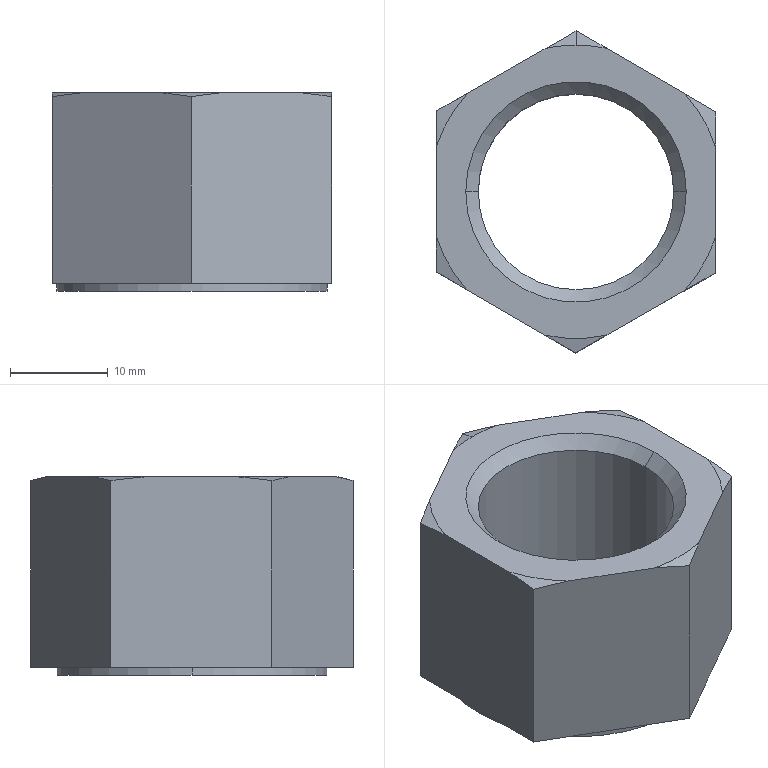Part | STEP file | 1 solid | 24 faces | box 28.6 x 32.95 x 20.3 mm | volume 7746 mm3 | cone 11 | plane 9 | cylinder 4 | commonest cylinder face diameters 20 x2 27.7 x2